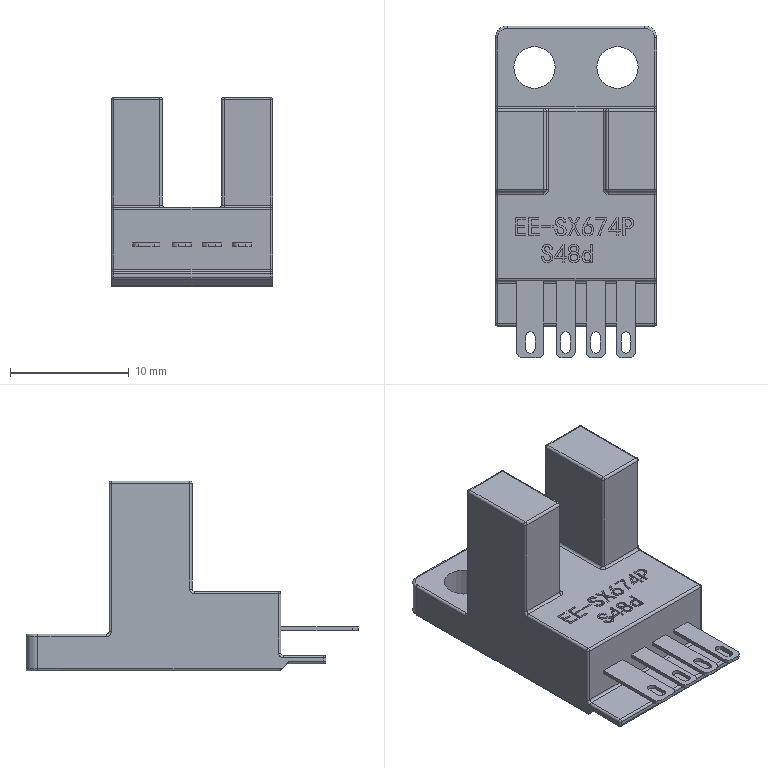Part | SolidWorks | features ICE 6, Fillet 3, Chamfer 1, Extrusion 1, HoleWzd 1 | 1 solid | 305 faces | box 13.6 x 28 x 16 mm | volume 2162 mm3 | plane 163 | cylinder 65 | spline 49 | sphere 14 | torus 14 | commonest cylinder face diameters 0.4 x43 0.8 x8 1 x8 3.5 x4 2 x2